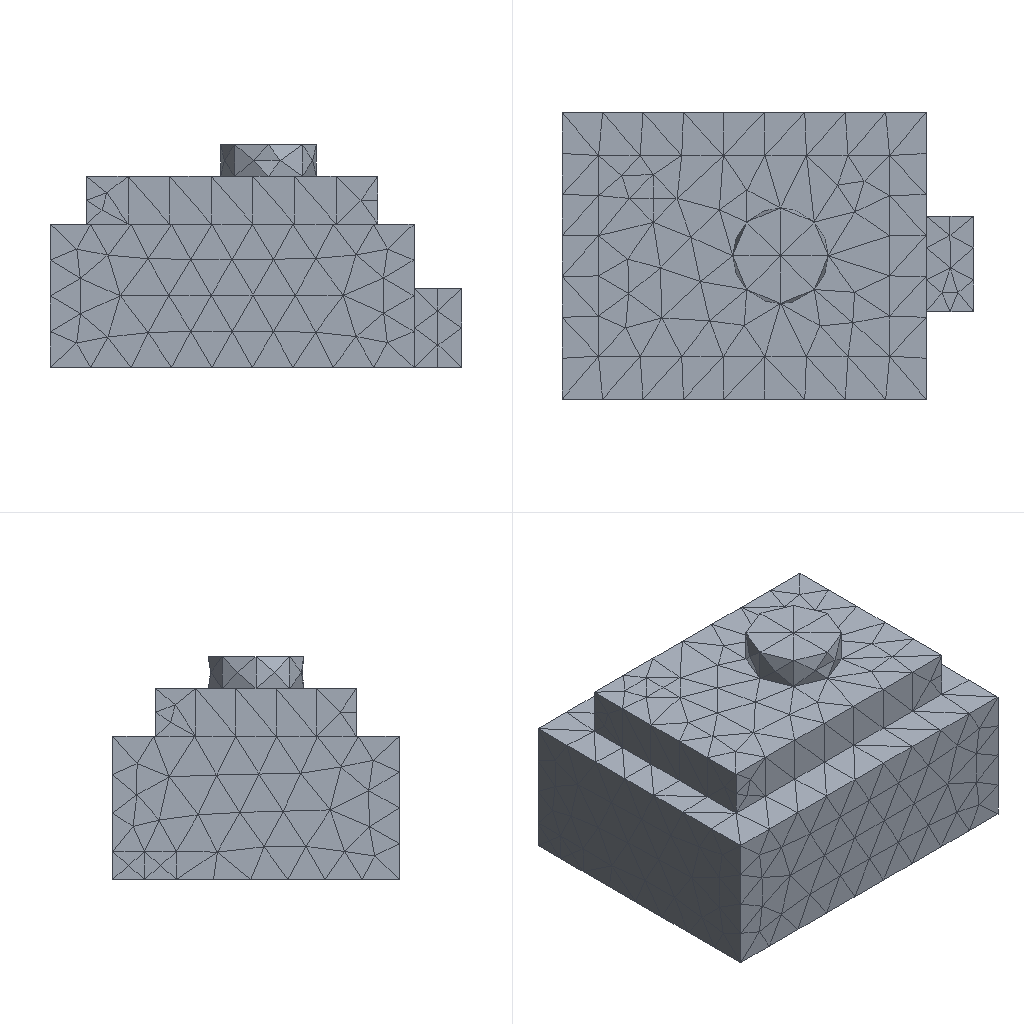Simulation study | ansys mapdl
Set-up summary:
category,name,step,type,value,unit,region
solver,ansys_mapdl
units,mm-N-s-tonne (MPa),,inferred,E=210000 density=
analysis,model,,static
mesh,nodes,,,4182
mesh,elements,,,2495
element_type,SOLID187,,,2495
material,mat 1,,E,210000
material,mat 1,,nu,0.3
load,,model,body load temp,,,all
load,,model,force,"1000 [dir=(0, 0, -1) n=318]",,node list
bc,,model,fixed,"[dofs=UX,UY,UZ n=4679]",,node list
Ansys APDL input file, long lists of numbers shortened:
/COM,ANSYS RELEASE 2026 R1           BUILD 26.1      UP20260202       09:09:40
/PREP7
/NOPR
/TITLE,2
ANTYPE, 0
*IF,_CDRDOFF,EQ,1,THEN     !if solid model was read in
_CDRDOFF=             !reset flag, numoffs already performed
*ELSE              !offset database for the following FE model
NUMOFF,NODE,     4182
NUMOFF,ELEM,     2495
NUMOFF,MAT ,        1
NUMOFF,TYPE,        1
*ENDIF
*SET,_RETURN ,  0.
*SET,_STATUS ,  0.
*SET,_UIQR   ,  318.
*SET,__FLOATPARAMETER__,  4182.
DOF,DELETE
ETBLOCK,        1,        1
(2i9,19a9)
        1      187        0        0        0        0        0        0        0        0        0        0        0        0        0        0        0        0        0        0        0
       -1
NBLOCK,6,SOLID,      4182,      4182
(3i9,6e21.13e3)
        1        0        0-2.9700000000000E+001 3.6000000000000E+001 7.0000000000000E+000
! (4181 more lines like these left out)
N,UNBL,LOC,       -1,
EBLOCK,19,SOLID,      2495,      2495
(19i10)
         1         1         1         1         0         0         0         0        10         0         1      1627      1341      1628      1354      1860      1861      1862      1863
! (4989 more lines like these left out)
        -1
MPTEMP,UNBL, 1, 1,  0.    ,
MPDATA,UNBL, 1,EX  ,       1, 1,  210000.000    ,
MPTEMP,UNBL, 1, 1,  0.    ,
MPDATA,UNBL, 1,NUXY,       1, 1, 0.3    ,
MPTEMP,UNBL, 1, 1,  0.    ,
MPDATA,UNBL, 1,PRXY,       1, 1, 0.3    ,
EXTOPT,ATTR,      0,      0,      0
EXTOPT,ESIZE,  0,  0.
EXTOPT,ACLEAR,      0
TREF,  0.
IRLF,  0
BFUNIF,TEMP,_TINY
ACEL,  0.    ,  0.    ,  0.
OMEGA,  0.    ,  0.    ,  0.
DOMEGA,  0.    ,  0.    ,  0.
CGLOC,  0.    ,  0.    ,  0.
CGOMEGA,  0.    ,  0.    ,  0.
DCGOMG,  0.    ,  0.    ,  0.
KUSE,     0
TIME,  0.
ALPHAD,  0.
BETAD,  0.
DMPRAT,  0.
DMPSTR,  0.
CRPLIM, 0.1    ,   0
CRPLIM,  0.    ,   1
NCNV,     0, 1.000000000E+12,     0,  0.    ,  0.
NEQIT,     0
ERESX,DEFA
DBLOCK,      4679
(i9,a6,2(pg16.9))
        1  UX    0.00000000      0.00000000
! (4678 more lines like these left out)
       -1
FBLOCK,       318
(i9,a6,2(pg16.9))
      532  FZ   -3.14465409      0.00000000
! (317 more lines like these left out)
       -1
/GO
FINISH
Results summary:
result,analysis_type_db,,,static,unstated
result,n_sets,,,1,unstated
result,load_steps[0].set,load_step=1,,1,unstated
result,load_steps[0].substep,load_step=1,,1,unstated
result,load_steps[0].time,load_step=1,,1,unstated
result,load_steps[0].freq,load_step=1,,1,unstated
result,load_steps[0].max_usum,load_step=1,,0.0001043,unstated
result,load_steps[0].max_seqv,load_step=1,,1.194,unstated
result,load_steps[0].reaction_sum.FX,load_step=1,,-5.62697e-12,unstated
result,load_steps[0].reaction_sum.FY,load_step=1,,1.40694e-11,unstated
result,load_steps[0].reaction_sum.FZ,load_step=1,,1000,unstated
result,load_steps[0].reaction_sum.MX,load_step=1,,0,unstated
result,load_steps[0].reaction_sum.MY,load_step=1,,0,unstated
result,load_steps[0].reaction_sum.MZ,load_step=1,,0,unstated
result,convergence,,,results present for all listed sets,unstated